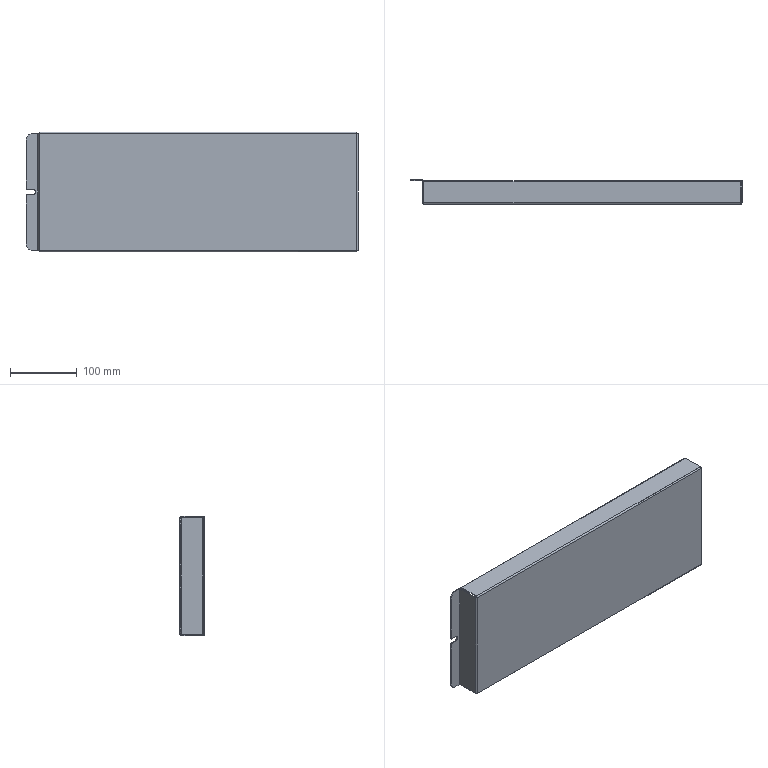Part | STEP file | 09-23 keyboard bracket (Default) | 1 solid | 81 faces | box 498.5 x 36.5 x 180 mm | volume 211119 mm3 | plane 45 | cylinder 28 | spline 8 | commonest cylinder face diameters 7 x8 1 x5 4 x5 15 x3 0.1 x2 3.1 x2